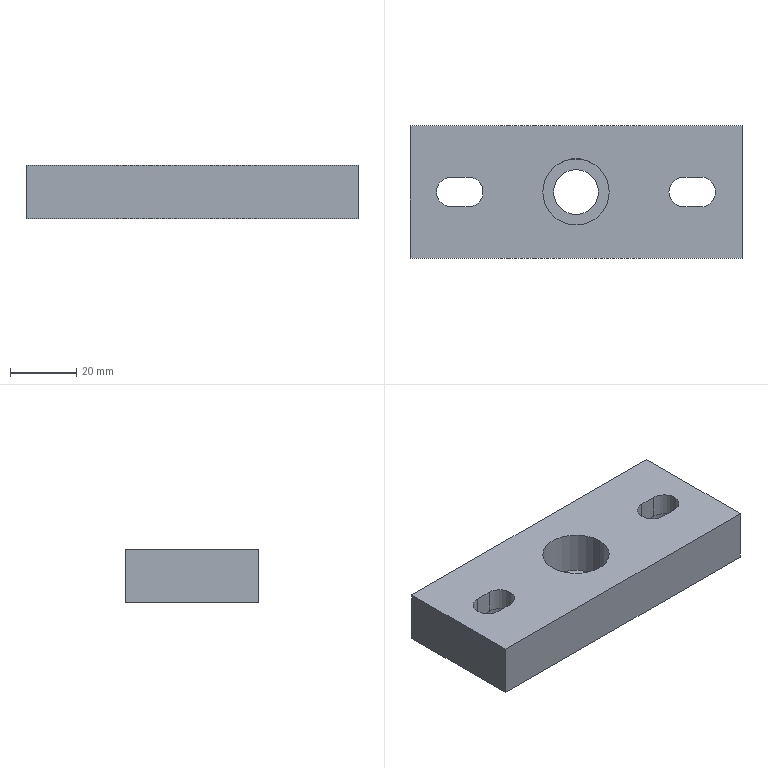Part | STEP file | X77b-01017 | 1 solid | 33 faces | box 100 x 40 x 16 mm | volume 53435 mm3 | plane 17 | cylinder 16 | commonest cylinder face diameters 9 x6 15 x6 13.5 x2 20 x2
STEP:
#1=CARTESIAN_POINT('',(10.527,125.181,9.));
#2=VERTEX_POINT('',#1);
#3=CARTESIAN_POINT('',(18.027,132.681,9.));
#4=VERTEX_POINT('',#3);
#5=CARTESIAN_POINT('',(18.027,125.181,9.));
#6=DIRECTION('',(0.,0.,-1.));
#7=DIRECTION('',(-1.,0.,0.));
#8=AXIS2_PLACEMENT_3D('',#5,#6,#7);
#9=CIRCLE('',#8,7.5);
#10=EDGE_CURVE('',#2,#4,#9,.T.);
#11=ORIENTED_EDGE('',*,*,#10,.F.);
#12=CARTESIAN_POINT('',(10.527,125.181,0.));
#13=VERTEX_POINT('',#12);
#14=CARTESIAN_POINT('',(10.527,125.181,9.));
#15=DIRECTION('',(0.,0.,-1.));
#16=VECTOR('',#15,1000.);
#17=LINE('',#14,#16);
#18=EDGE_CURVE('',#2,#13,#17,.T.);
#19=ORIENTED_EDGE('',*,*,#18,.T.);
#20=CARTESIAN_POINT('',(18.027,132.681,0.));
#21=VERTEX_POINT('',#20);
#22=CARTESIAN_POINT('',(18.027,125.181,0.));
#23=DIRECTION('',(0.,0.,-1.));
#24=DIRECTION('',(-1.,0.,0.));
#25=AXIS2_PLACEMENT_3D('',#22,#23,#24);
#26=CIRCLE('',#25,7.5);
#27=EDGE_CURVE('',#13,#21,#26,.T.);
#28=ORIENTED_EDGE('',*,*,#27,.T.);
#29=CARTESIAN_POINT('',(18.027,132.681,9.));
#30=DIRECTION('',(0.,0.,-1.));
#31=VECTOR('',#30,1000.);
#32=LINE('',#29,#31);
#33=EDGE_CURVE('',#4,#21,#32,.T.);
#34=ORIENTED_EDGE('',*,*,#33,.F.);
#35=EDGE_LOOP('',(#11,#19,#28,#34));
#36=FACE_OUTER_BOUND('',#35,.T.);
#37=CARTESIAN_POINT('',(18.027,125.181,9.));
#38=DIRECTION('',(0.,0.,-1.));
#39=DIRECTION('',(-1.,0.,0.));
#40=AXIS2_PLACEMENT_3D('',#37,#38,#39);
#41=CYLINDRICAL_SURFACE('',#40,7.5);
#42=ADVANCED_FACE('',(#36),#41,.F.);
#43=CARTESIAN_POINT('',(-59.473,125.181,9.));
#44=VERTEX_POINT('',#43);
#45=CARTESIAN_POINT('',(-51.973,132.681,9.));
#46=VERTEX_POINT('',#45);
#47=CARTESIAN_POINT('',(-51.973,125.181,9.));
#48=DIRECTION('',(0.,0.,-1.));
#49=DIRECTION('',(-1.,0.,0.));
#50=AXIS2_PLACEMENT_3D('',#47,#48,#49);
#51=CIRCLE('',#50,7.5);
#52=EDGE_CURVE('',#44,#46,#51,.T.);
#53=ORIENTED_EDGE('',*,*,#52,.F.);
#54=CARTESIAN_POINT('',(-59.473,125.181,0.));
#55=VERTEX_POINT('',#54);
#56=CARTESIAN_POINT('',(-59.473,125.181,9.));
#57=DIRECTION('',(0.,0.,-1.));
#58=VECTOR('',#57,1000.);
#59=LINE('',#56,#58);
#60=EDGE_CURVE('',#44,#55,#59,.T.);
#61=ORIENTED_EDGE('',*,*,#60,.T.);
#62=CARTESIAN_POINT('',(-51.973,132.681,0.));
#63=VERTEX_POINT('',#62);
#64=CARTESIAN_POINT('',(-51.973,125.181,0.));
#65=DIRECTION('',(0.,0.,-1.));
#66=DIRECTION('',(-1.,0.,0.));
#67=AXIS2_PLACEMENT_3D('',#64,#65,#66);
#68=CIRCLE('',#67,7.5);
#69=EDGE_CURVE('',#55,#63,#68,.T.);
#70=ORIENTED_EDGE('',*,*,#69,.T.);
#71=CARTESIAN_POINT('',(-51.973,132.681,9.));
#72=DIRECTION('',(0.,0.,-1.));
#73=VECTOR('',#72,1000.);
#74=LINE('',#71,#73);
#75=EDGE_CURVE('',#46,#63,#74,.T.);
#76=ORIENTED_EDGE('',*,*,#75,.F.);
#77=EDGE_LOOP('',(#53,#61,#70,#76));
#78=FACE_OUTER_BOUND('',#77,.T.);
#79=CARTESIAN_POINT('',(-51.973,125.181,9.));
#80=DIRECTION('',(0.,0.,-1.));
#81=DIRECTION('',(-1.,0.,0.));
#82=AXIS2_PLACEMENT_3D('',#79,#80,#81);
#83=CYLINDRICAL_SURFACE('',#82,7.5);
#84=ADVANCED_FACE('',(#78),#83,.F.);
#85=CARTESIAN_POINT('',(-24.473,125.181,3.));
#86=VERTEX_POINT('',#85);
#87=CARTESIAN_POINT('',(-4.473,125.181,3.));
#88=VERTEX_POINT('',#87);
#89=CARTESIAN_POINT('',(-14.473,125.181,3.));
#90=DIRECTION('',(0.,0.,1.));
#91=DIRECTION('',(1.,0.,0.));
#92=AXIS2_PLACEMENT_3D('',#89,#90,#91);
#93=CIRCLE('',#92,10.);
#94=EDGE_CURVE('',#86,#88,#93,.T.);
#95=ORIENTED_EDGE('',*,*,#94,.F.);
#96=CARTESIAN_POINT('',(-24.473,125.181,16.));
#97=VERTEX_POINT('',#96);
#98=CARTESIAN_POINT('',(-24.473,125.181,16.));
#99=DIRECTION('',(0.,0.,1.));
#100=VECTOR('',#99,1000.);
#101=LINE('',#98,#100);
#102=EDGE_CURVE('',#86,#97,#101,.T.);
#103=ORIENTED_EDGE('',*,*,#102,.T.);
#104=CARTESIAN_POINT('',(-4.473,125.181,16.));
#105=VERTEX_POINT('',#104);
#106=CARTESIAN_POINT('',(-14.473,125.181,16.));
#107=DIRECTION('',(0.,0.,1.));
#108=DIRECTION('',(1.,0.,0.));
#109=AXIS2_PLACEMENT_3D('',#106,#107,#108);
#110=CIRCLE('',#109,10.);
#111=EDGE_CURVE('',#97,#105,#110,.T.);
#112=ORIENTED_EDGE('',*,*,#111,.T.);
#113=CARTESIAN_POINT('',(-4.473,125.181,16.));
#114=DIRECTION('',(0.,0.,1.));
#115=VECTOR('',#114,1000.);
#116=LINE('',#113,#115);
#117=EDGE_CURVE('',#88,#105,#116,.T.);
#118=ORIENTED_EDGE('',*,*,#117,.F.);
#119=EDGE_LOOP('',(#95,#103,#112,#118));
#120=FACE_OUTER_BOUND('',#119,.T.);
#121=CARTESIAN_POINT('',(-14.473,125.181,16.));
#122=DIRECTION('',(0.,0.,1.));
#123=DIRECTION('',(1.,0.,0.));
#124=AXIS2_PLACEMENT_3D('',#121,#122,#123);
#125=CYLINDRICAL_SURFACE('',#124,10.);
#126=ADVANCED_FACE('',(#120),#125,.F.);
#127=CARTESIAN_POINT('',(-21.223,125.181,0.));
#128=VERTEX_POINT('',#127);
#129=CARTESIAN_POINT('',(-7.723,125.181,0.));
#130=VERTEX_POINT('',#129);
#131=CARTESIAN_POINT('',(-14.473,125.181,0.));
#132=DIRECTION('',(0.,0.,1.));
#133=DIRECTION('',(1.,0.,0.));
#134=AXIS2_PLACEMENT_3D('',#131,#132,#133);
#135=CIRCLE('',#134,6.75);
#136=EDGE_CURVE('',#128,#130,#135,.T.);
#137=ORIENTED_EDGE('',*,*,#136,.F.);
#138=CARTESIAN_POINT('',(-21.223,125.181,3.));
#139=VERTEX_POINT('',#138);
#140=CARTESIAN_POINT('',(-21.223,125.181,16.));
#141=DIRECTION('',(0.,0.,1.));
#142=VECTOR('',#141,1000.);
#143=LINE('',#140,#142);
#144=EDGE_CURVE('',#128,#139,#143,.T.);
#145=ORIENTED_EDGE('',*,*,#144,.T.);
#146=CARTESIAN_POINT('',(-7.723,125.181,3.));
#147=VERTEX_POINT('',#146);
#148=CARTESIAN_POINT('',(-14.473,125.181,3.));
#149=DIRECTION('',(0.,0.,1.));
#150=DIRECTION('',(1.,0.,0.));
#151=AXIS2_PLACEMENT_3D('',#148,#149,#150);
#152=CIRCLE('',#151,6.75);
#153=EDGE_CURVE('',#139,#147,#152,.T.);
#154=ORIENTED_EDGE('',*,*,#153,.T.);
#155=CARTESIAN_POINT('',(-7.723,125.181,16.));
#156=DIRECTION('',(0.,0.,1.));
#157=VECTOR('',#156,1000.);
#158=LINE('',#155,#157);
#159=EDGE_CURVE('',#130,#147,#158,.T.);
#160=ORIENTED_EDGE('',*,*,#159,.F.);
#161=EDGE_LOOP('',(#137,#145,#154,#160));
#162=FACE_OUTER_BOUND('',#161,.T.);
#163=CARTESIAN_POINT('',(-14.473,125.181,16.));
#164=DIRECTION('',(0.,0.,1.));
#165=DIRECTION('',(1.,0.,0.));
#166=AXIS2_PLACEMENT_3D('',#163,#164,#165);
#167=CYLINDRICAL_SURFACE('',#166,6.75);
#168=ADVANCED_FACE('',(#162),#167,.F.);
#169=CARTESIAN_POINT('',(-56.473,125.181,16.));
#170=VERTEX_POINT('',#169);
#171=CARTESIAN_POINT('',(-51.973,129.681,16.));
#172=VERTEX_POINT('',#171);
#173=CARTESIAN_POINT('',(-51.973,125.181,16.));
#174=DIRECTION('',(0.,0.,-1.));
#175=DIRECTION('',(-1.,0.,0.));
#176=AXIS2_PLACEMENT_3D('',#173,#174,#175);
#177=CIRCLE('',#176,4.5);
#178=EDGE_CURVE('',#170,#172,#177,.T.);
#179=ORIENTED_EDGE('',*,*,#178,.F.);
#180=CARTESIAN_POINT('',(-56.473,125.181,9.));
#181=VERTEX_POINT('',#180);
#182=CARTESIAN_POINT('',(-56.473,125.181,16.));
#183=DIRECTION('',(0.,0.,-1.));
#184=VECTOR('',#183,1000.);
#185=LINE('',#182,#184);
#186=EDGE_CURVE('',#170,#181,#185,.T.);
#187=ORIENTED_EDGE('',*,*,#186,.T.);
#188=CARTESIAN_POINT('',(-51.973,129.681,9.));
#189=VERTEX_POINT('',#188);
#190=CARTESIAN_POINT('',(-51.973,125.181,9.));
#191=DIRECTION('',(0.,0.,1.));
#192=DIRECTION('',(-1.,0.,0.));
#193=AXIS2_PLACEMENT_3D('',#190,#191,#192);
#194=CIRCLE('',#193,4.5);
#195=EDGE_CURVE('',#189,#181,#194,.T.);
#196=ORIENTED_EDGE('',*,*,#195,.F.);
#197=CARTESIAN_POINT('',(-51.973,129.681,16.));
#198=DIRECTION('',(0.,0.,-1.));
#199=VECTOR('',#198,1000.);
#200=LINE('',#197,#199);
#201=EDGE_CURVE('',#172,#189,#200,.T.);
#202=ORIENTED_EDGE('',*,*,#201,.F.);
#203=EDGE_LOOP('',(#179,#187,#196,#202));
#204=FACE_OUTER_BOUND('',#203,.T.);
#205=CARTESIAN_POINT('',(-51.973,125.181,16.));
#206=DIRECTION('',(0.,0.,-1.));
#207=DIRECTION('',(-1.,0.,0.));
#208=AXIS2_PLACEMENT_3D('',#205,#206,#207);
#209=CYLINDRICAL_SURFACE('',#208,4.5);
#210=ADVANCED_FACE('',(#204),#209,.F.);
#211=CARTESIAN_POINT('',(13.527,125.181,16.));
#212=VERTEX_POINT('',#211);
#213=CARTESIAN_POINT('',(18.027,129.681,16.));
#214=VERTEX_POINT('',#213);
#215=CARTESIAN_POINT('',(18.027,125.181,16.));
#216=DIRECTION('',(0.,0.,-1.));
#217=DIRECTION('',(-1.,0.,0.));
#218=AXIS2_PLACEMENT_3D('',#215,#216,#217);
#219=CIRCLE('',#218,4.5);
#220=EDGE_CURVE('',#212,#214,#219,.T.);
#221=ORIENTED_EDGE('',*,*,#220,.F.);
#222=CARTESIAN_POINT('',(13.527,125.181,9.));
#223=VERTEX_POINT('',#222);
#224=CARTESIAN_POINT('',(13.527,125.181,16.));
#225=DIRECTION('',(0.,0.,-1.));
#226=VECTOR('',#225,1000.);
#227=LINE('',#224,#226);
#228=EDGE_CURVE('',#212,#223,#227,.T.);
#229=ORIENTED_EDGE('',*,*,#228,.T.);
#230=CARTESIAN_POINT('',(18.027,129.681,9.));
#231=VERTEX_POINT('',#230);
#232=CARTESIAN_POINT('',(18.027,125.181,9.));
#233=DIRECTION('',(0.,0.,1.));
#234=DIRECTION('',(-1.,0.,0.));
#235=AXIS2_PLACEMENT_3D('',#232,#233,#234);
#236=CIRCLE('',#235,4.5);
#237=EDGE_CURVE('',#231,#223,#236,.T.);
#238=ORIENTED_EDGE('',*,*,#237,.F.);
#239=CARTESIAN_POINT('',(18.027,129.681,16.));
#240=DIRECTION('',(0.,0.,-1.));
#241=VECTOR('',#240,1000.);
#242=LINE('',#239,#241);
#243=EDGE_CURVE('',#214,#231,#242,.T.);
#244=ORIENTED_EDGE('',*,*,#243,.F.);
#245=EDGE_LOOP('',(#221,#229,#238,#244));
#246=FACE_OUTER_BOUND('',#245,.T.);
#247=CARTESIAN_POINT('',(18.027,125.181,16.));
#248=DIRECTION('',(0.,0.,-1.));
#249=DIRECTION('',(-1.,0.,0.));
#250=AXIS2_PLACEMENT_3D('',#247,#248,#249);
#251=CYLINDRICAL_SURFACE('',#250,4.5);
#252=ADVANCED_FACE('',(#246),#251,.F.);
#253=CARTESIAN_POINT('',(23.027,120.681,9.));
#254=VERTEX_POINT('',#253);
#255=CARTESIAN_POINT('',(23.027,129.681,9.));
#256=VERTEX_POINT('',#255);
#257=CARTESIAN_POINT('',(23.027,125.181,9.));
#258=DIRECTION('',(0.,0.,1.));
#259=DIRECTION('',(-1.,0.,0.));
#260=AXIS2_PLACEMENT_3D('',#257,#258,#259);
#261=CIRCLE('',#260,4.5);
#262=EDGE_CURVE('',#254,#256,#261,.T.);
#263=ORIENTED_EDGE('',*,*,#262,.F.);
#264=CARTESIAN_POINT('',(23.027,120.681,16.));
#265=VERTEX_POINT('',#264);
#266=CARTESIAN_POINT('',(23.027,120.681,16.));
#267=DIRECTION('',(0.,0.,-1.));
#268=VECTOR('',#267,1000.);
#269=LINE('',#266,#268);
#270=EDGE_CURVE('',#265,#254,#269,.T.);
#271=ORIENTED_EDGE('',*,*,#270,.F.);
#272=CARTESIAN_POINT('',(23.027,129.681,16.));
#273=VERTEX_POINT('',#272);
#274=CARTESIAN_POINT('',(23.027,125.181,16.));
#275=DIRECTION('',(0.,0.,-1.));
#276=DIRECTION('',(-1.,0.,0.));
#277=AXIS2_PLACEMENT_3D('',#274,#275,#276);
#278=CIRCLE('',#277,4.5);
#279=EDGE_CURVE('',#273,#265,#278,.T.);
#280=ORIENTED_EDGE('',*,*,#279,.F.);
#281=CARTESIAN_POINT('',(23.027,129.681,16.));
#282=DIRECTION('',(0.,0.,-1.));
#283=VECTOR('',#282,1000.);
#284=LINE('',#281,#283);
#285=EDGE_CURVE('',#273,#256,#284,.T.);
#286=ORIENTED_EDGE('',*,*,#285,.T.);
#287=EDGE_LOOP('',(#263,#271,#280,#286));
#288=FACE_OUTER_BOUND('',#287,.T.);
#289=CARTESIAN_POINT('',(23.027,125.181,16.));
#290=DIRECTION('',(0.,0.,-1.));
#291=DIRECTION('',(-1.,0.,0.));
#292=AXIS2_PLACEMENT_3D('',#289,#290,#291);
#293=CYLINDRICAL_SURFACE('',#292,4.5);
#294=ADVANCED_FACE('',(#288),#293,.F.);
#295=CARTESIAN_POINT('',(23.027,129.681,9.));
#296=DIRECTION('',(-1.,0.,0.));
#297=VECTOR('',#296,1000.);
#298=LINE('',#295,#297);
#299=EDGE_CURVE('',#256,#231,#298,.T.);
#300=ORIENTED_EDGE('',*,*,#299,.F.);
#301=ORIENTED_EDGE('',*,*,#285,.F.);
#302=CARTESIAN_POINT('',(23.027,129.681,16.));
#303=DIRECTION('',(1.,0.,0.));
#304=VECTOR('',#303,1000.);
#305=LINE('',#302,#304);
#306=EDGE_CURVE('',#214,#273,#305,.T.);
#307=ORIENTED_EDGE('',*,*,#306,.F.);
#308=ORIENTED_EDGE('',*,*,#243,.T.);
#309=EDGE_LOOP('',(#300,#301,#307,#308));
#310=FACE_OUTER_BOUND('',#309,.T.);
#311=CARTESIAN_POINT('',(23.027,129.681,16.));
#312=DIRECTION('',(0.,1.,0.));
#313=DIRECTION('',(0.,0.,1.));
#314=AXIS2_PLACEMENT_3D('',#311,#312,#313);
#315=PLANE('',#314);
#316=ADVANCED_FACE('',(#310),#315,.F.);
#317=ORIENTED_EDGE('',*,*,#228,.F.);
#318=CARTESIAN_POINT('',(18.027,120.681,16.));
#319=VERTEX_POINT('',#318);
#320=CARTESIAN_POINT('',(18.027,125.181,16.));
#321=DIRECTION('',(0.,0.,-1.));
#322=DIRECTION('',(-1.,0.,0.));
#323=AXIS2_PLACEMENT_3D('',#320,#321,#322);
#324=CIRCLE('',#323,4.5);
#325=EDGE_CURVE('',#319,#212,#324,.T.);
#326=ORIENTED_EDGE('',*,*,#325,.F.);
#327=CARTESIAN_POINT('',(18.027,120.681,9.));
#328=VERTEX_POINT('',#327);
#329=CARTESIAN_POINT('',(18.027,120.681,16.));
#330=DIRECTION('',(0.,0.,-1.));
#331=VECTOR('',#330,1000.);
#332=LINE('',#329,#331);
#333=EDGE_CURVE('',#319,#328,#332,.T.);
#334=ORIENTED_EDGE('',*,*,#333,.T.);
#335=CARTESIAN_POINT('',(18.027,125.181,9.));
#336=DIRECTION('',(0.,0.,1.));
#337=DIRECTION('',(-1.,0.,0.));
#338=AXIS2_PLACEMENT_3D('',#335,#336,#337);
#339=CIRCLE('',#338,4.5);
#340=EDGE_CURVE('',#223,#328,#339,.T.);
#341=ORIENTED_EDGE('',*,*,#340,.F.);
#342=EDGE_LOOP('',(#317,#326,#334,#341));
#343=FACE_OUTER_BOUND('',#342,.T.);
#344=CARTESIAN_POINT('',(18.027,125.181,16.));
#345=DIRECTION('',(0.,0.,-1.));
#346=DIRECTION('',(-1.,0.,0.));
#347=AXIS2_PLACEMENT_3D('',#344,#345,#346);
#348=CYLINDRICAL_SURFACE('',#347,4.5);
#349=ADVANCED_FACE('',(#343),#348,.F.);
#350=CARTESIAN_POINT('',(23.027,120.681,9.));
#351=DIRECTION('',(1.,0.,0.));
#352=VECTOR('',#351,1000.);
#353=LINE('',#350,#352);
#354=EDGE_CURVE('',#328,#254,#353,.T.);
#355=ORIENTED_EDGE('',*,*,#354,.F.);
#356=ORIENTED_EDGE('',*,*,#333,.F.);
#357=CARTESIAN_POINT('',(23.027,120.681,16.));
#358=DIRECTION('',(-1.,0.,0.));
#359=VECTOR('',#358,1000.);
#360=LINE('',#357,#359);
#361=EDGE_CURVE('',#265,#319,#360,.T.);
#362=ORIENTED_EDGE('',*,*,#361,.F.);
#363=ORIENTED_EDGE('',*,*,#270,.T.);
#364=EDGE_LOOP('',(#355,#356,#362,#363));
#365=FACE_OUTER_BOUND('',#364,.T.);
#366=CARTESIAN_POINT('',(23.027,120.681,16.));
#367=DIRECTION('',(0.,-1.,0.));
#368=DIRECTION('',(0.,0.,-1.));
#369=AXIS2_PLACEMENT_3D('',#366,#367,#368);
#370=PLANE('',#369);
#371=ADVANCED_FACE('',(#365),#370,.F.);
#372=CARTESIAN_POINT('',(-46.973,120.681,9.));
#373=VERTEX_POINT('',#372);
#374=CARTESIAN_POINT('',(-46.973,129.681,9.));
#375=VERTEX_POINT('',#374);
#376=CARTESIAN_POINT('',(-46.973,125.181,9.));
#377=DIRECTION('',(0.,0.,1.));
#378=DIRECTION('',(-1.,0.,0.));
#379=AXIS2_PLACEMENT_3D('',#376,#377,#378);
#380=CIRCLE('',#379,4.5);
#381=EDGE_CURVE('',#373,#375,#380,.T.);
#382=ORIENTED_EDGE('',*,*,#381,.F.);
#383=CARTESIAN_POINT('',(-46.973,120.681,16.));
#384=VERTEX_POINT('',#383);
#385=CARTESIAN_POINT('',(-46.973,120.681,16.));
#386=DIRECTION('',(0.,0.,-1.));
#387=VECTOR('',#386,1000.);
#388=LINE('',#385,#387);
#389=EDGE_CURVE('',#384,#373,#388,.T.);
#390=ORIENTED_EDGE('',*,*,#389,.F.);
#391=CARTESIAN_POINT('',(-46.973,129.681,16.));
#392=VERTEX_POINT('',#391);
#393=CARTESIAN_POINT('',(-46.973,125.181,16.));
#394=DIRECTION('',(0.,0.,-1.));
#395=DIRECTION('',(-1.,0.,0.));
#396=AXIS2_PLACEMENT_3D('',#393,#394,#395);
#397=CIRCLE('',#396,4.5);
#398=EDGE_CURVE('',#392,#384,#397,.T.);
#399=ORIENTED_EDGE('',*,*,#398,.F.);
#400=CARTESIAN_POINT('',(-46.973,129.681,16.));
#401=DIRECTION('',(0.,0.,-1.));
#402=VECTOR('',#401,1000.);
#403=LINE('',#400,#402);
#404=EDGE_CURVE('',#392,#375,#403,.T.);
#405=ORIENTED_EDGE('',*,*,#404,.T.);
#406=EDGE_LOOP('',(#382,#390,#399,#405));
#407=FACE_OUTER_BOUND('',#406,.T.);
#408=CARTESIAN_POINT('',(-46.973,125.181,16.));
#409=DIRECTION('',(0.,0.,-1.));
#410=DIRECTION('',(-1.,0.,0.));
#411=AXIS2_PLACEMENT_3D('',#408,#409,#410);
#412=CYLINDRICAL_SURFACE('',#411,4.5);
#413=ADVANCED_FACE('',(#407),#412,.F.);
#414=CARTESIAN_POINT('',(-46.973,129.681,9.));
#415=DIRECTION('',(-1.,0.,0.));
#416=VECTOR('',#415,1000.);
#417=LINE('',#414,#416);
#418=EDGE_CURVE('',#375,#189,#417,.T.);
#419=ORIENTED_EDGE('',*,*,#418,.F.);
#420=ORIENTED_EDGE('',*,*,#404,.F.);
#421=CARTESIAN_POINT('',(-46.973,129.681,16.));
#422=DIRECTION('',(1.,0.,0.));
#423=VECTOR('',#422,1000.);
#424=LINE('',#421,#423);
#425=EDGE_CURVE('',#172,#392,#424,.T.);
#426=ORIENTED_EDGE('',*,*,#425,.F.);
#427=ORIENTED_EDGE('',*,*,#201,.T.);
#428=EDGE_LOOP('',(#419,#420,#426,#427));
#429=FACE_OUTER_BOUND('',#428,.T.);
#430=CARTESIAN_POINT('',(-46.973,129.681,16.));
#431=DIRECTION('',(0.,1.,0.));
#432=DIRECTION('',(0.,0.,1.));
#433=AXIS2_PLACEMENT_3D('',#430,#431,#432);
#434=PLANE('',#433);
#435=ADVANCED_FACE('',(#429),#434,.F.);
#436=ORIENTED_EDGE('',*,*,#186,.F.);
#437=CARTESIAN_POINT('',(-51.973,120.681,16.));
#438=VERTEX_POINT('',#437);
#439=CARTESIAN_POINT('',(-51.973,125.181,16.));
#440=DIRECTION('',(0.,0.,-1.));
#441=DIRECTION('',(-1.,0.,0.));
#442=AXIS2_PLACEMENT_3D('',#439,#440,#441);
#443=CIRCLE('',#442,4.5);
#444=EDGE_CURVE('',#438,#170,#443,.T.);
#445=ORIENTED_EDGE('',*,*,#444,.F.);
#446=CARTESIAN_POINT('',(-51.973,120.681,9.));
#447=VERTEX_POINT('',#446);
#448=CARTESIAN_POINT('',(-51.973,120.681,16.));
#449=DIRECTION('',(0.,0.,-1.));
#450=VECTOR('',#449,1000.);
#451=LINE('',#448,#450);
#452=EDGE_CURVE('',#438,#447,#451,.T.);
#453=ORIENTED_EDGE('',*,*,#452,.T.);
#454=CARTESIAN_POINT('',(-51.973,125.181,9.));
#455=DIRECTION('',(0.,0.,1.));
#456=DIRECTION('',(-1.,0.,0.));
#457=AXIS2_PLACEMENT_3D('',#454,#455,#456);
#458=CIRCLE('',#457,4.5);
#459=EDGE_CURVE('',#181,#447,#458,.T.);
#460=ORIENTED_EDGE('',*,*,#459,.F.);
#461=EDGE_LOOP('',(#436,#445,#453,#460));
#462=FACE_OUTER_BOUND('',#461,.T.);
#463=CARTESIAN_POINT('',(-51.973,125.181,16.));
#464=DIRECTION('',(0.,0.,-1.));
#465=DIRECTION('',(-1.,0.,0.));
#466=AXIS2_PLACEMENT_3D('',#463,#464,#465);
#467=CYLINDRICAL_SURFACE('',#466,4.5);
#468=ADVANCED_FACE('',(#462),#467,.F.);
#469=CARTESIAN_POINT('',(-46.973,120.681,9.));
#470=DIRECTION('',(1.,0.,0.));
#471=VECTOR('',#470,1000.);
#472=LINE('',#469,#471);
#473=EDGE_CURVE('',#447,#373,#472,.T.);
#474=ORIENTED_EDGE('',*,*,#473,.F.);
#475=ORIENTED_EDGE('',*,*,#452,.F.);
#476=CARTESIAN_POINT('',(-46.973,120.681,16.));
#477=DIRECTION('',(-1.,0.,0.));
#478=VECTOR('',#477,1000.);
#479=LINE('',#476,#478);
#480=EDGE_CURVE('',#384,#438,#479,.T.);
#481=ORIENTED_EDGE('',*,*,#480,.F.);
#482=ORIENTED_EDGE('',*,*,#389,.T.);
#483=EDGE_LOOP('',(#474,#475,#481,#482));
#484=FACE_OUTER_BOUND('',#483,.T.);
#485=CARTESIAN_POINT('',(-46.973,120.681,16.));
#486=DIRECTION('',(0.,-1.,0.));
#487=DIRECTION('',(0.,0.,-1.));
#488=AXIS2_PLACEMENT_3D('',#485,#486,#487);
#489=PLANE('',#488);
#490=ADVANCED_FACE('',(#484),#489,.F.);
#491=CARTESIAN_POINT('',(-64.473,145.181,0.));
#492=VERTEX_POINT('',#491);
#493=CARTESIAN_POINT('',(-64.473,105.181,0.));
#494=VERTEX_POINT('',#493);
#495=CARTESIAN_POINT('',(-64.473,105.181,0.));
#496=DIRECTION('',(0.,-1.,0.));
#497=VECTOR('',#496,1000.);
#498=LINE('',#495,#497);
#499=EDGE_CURVE('',#492,#494,#498,.T.);
#500=ORIENTED_EDGE('',*,*,#499,.T.);
#501=CARTESIAN_POINT('',(-64.473,105.181,16.));
#502=VERTEX_POINT('',#501);
#503=CARTESIAN_POINT('',(-64.473,105.181,16.));
#504=DIRECTION('',(0.,0.,-1.));
#505=VECTOR('',#504,1000.);
#506=LINE('',#503,#505);
#507=EDGE_CURVE('',#502,#494,#506,.T.);
#508=ORIENTED_EDGE('',*,*,#507,.F.);
#509=CARTESIAN_POINT('',(-64.473,145.181,16.));
#510=VERTEX_POINT('',#509);
#511=CARTESIAN_POINT('',(-64.473,105.181,16.));
#512=DIRECTION('',(0.,-1.,0.));
#513=VECTOR('',#512,1000.);
#514=LINE('',#511,#513);
#515=EDGE_CURVE('',#510,#502,#514,.T.);
#516=ORIENTED_EDGE('',*,*,#515,.F.);
#517=CARTESIAN_POINT('',(-64.473,145.181,16.));
#518=DIRECTION('',(0.,0.,-1.));
#519=VECTOR('',#518,1000.);
#520=LINE('',#517,#519);
#521=EDGE_CURVE('',#510,#492,#520,.T.);
#522=ORIENTED_EDGE('',*,*,#521,.T.);
#523=EDGE_LOOP('',(#500,#508,#516,#522));
#524=FACE_OUTER_BOUND('',#523,.T.);
#525=CARTESIAN_POINT('',(-64.473,105.181,16.));
#526=DIRECTION('',(1.,0.,0.));
#527=DIRECTION('',(0.,0.,-1.));
#528=AXIS2_PLACEMENT_3D('',#525,#526,#527);
#529=PLANE('',#528);
#530=ADVANCED_FACE('',(#524),#529,.F.);
#531=CARTESIAN_POINT('',(35.527,105.181,0.));
#532=VERTEX_POINT('',#531);
#533=CARTESIAN_POINT('',(-64.473,105.181,0.));
#534=DIRECTION('',(1.,0.,0.));
#535=VECTOR('',#534,1000.);
#536=LINE('',#533,#535);
#537=EDGE_CURVE('',#494,#532,#536,.T.);
#538=ORIENTED_EDGE('',*,*,#537,.T.);
#539=CARTESIAN_POINT('',(35.527,105.181,16.));
#540=VERTEX_POINT('',#539);
#541=CARTESIAN_POINT('',(35.527,105.181,16.));
#542=DIRECTION('',(0.,0.,-1.));
#543=VECTOR('',#542,1000.);
#544=LINE('',#541,#543);
#545=EDGE_CURVE('',#540,#532,#544,.T.);
#546=ORIENTED_EDGE('',*,*,#545,.F.);
#547=CARTESIAN_POINT('',(-64.473,105.181,16.));
#548=DIRECTION('',(1.,0.,0.));
#549=VECTOR('',#548,1000.);
#550=LINE('',#547,#549);
#551=EDGE_CURVE('',#502,#540,#550,.T.);
#552=ORIENTED_EDGE('',*,*,#551,.F.);
#553=ORIENTED_EDGE('',*,*,#507,.T.);
#554=EDGE_LOOP('',(#538,#546,#552,#553));
#555=FACE_OUTER_BOUND('',#554,.T.);
#556=CARTESIAN_POINT('',(-64.473,105.181,16.));
#557=DIRECTION('',(0.,1.,0.));
#558=DIRECTION('',(0.,0.,1.));
#559=AXIS2_PLACEMENT_3D('',#556,#557,#558);
#560=PLANE('',#559);
#561=ADVANCED_FACE('',(#555),#560,.F.);
#562=CARTESIAN_POINT('',(35.527,145.181,0.));
#563=VERTEX_POINT('',#562);
#564=CARTESIAN_POINT('',(35.527,105.181,0.));
#565=DIRECTION('',(0.,1.,0.));
#566=VECTOR('',#565,1000.);
#567=LINE('',#564,#566);
#568=EDGE_CURVE('',#532,#563,#567,.T.);
#569=ORIENTED_EDGE('',*,*,#568,.T.);
#570=CARTESIAN_POINT('',(35.527,145.181,16.));
#571=VERTEX_POINT('',#570);
#572=CARTESIAN_POINT('',(35.527,145.181,16.));
#573=DIRECTION('',(0.,0.,-1.));
#574=VECTOR('',#573,1000.);
#575=LINE('',#572,#574);
#576=EDGE_CURVE('',#571,#563,#575,.T.);
#577=ORIENTED_EDGE('',*,*,#576,.F.);
#578=CARTESIAN_POINT('',(35.527,105.181,16.));
#579=DIRECTION('',(0.,1.,0.));
#580=VECTOR('',#579,1000.);
#581=LINE('',#578,#580);
#582=EDGE_CURVE('',#540,#571,#581,.T.);
#583=ORIENTED_EDGE('',*,*,#582,.F.);
#584=ORIENTED_EDGE('',*,*,#545,.T.);
#585=EDGE_LOOP('',(#569,#577,#583,#584));
#586=FACE_OUTER_BOUND('',#585,.T.);
#587=CARTESIAN_POINT('',(35.527,105.181,16.));
#588=DIRECTION('',(-1.,0.,0.));
#589=DIRECTION('',(0.,0.,1.));
#590=AXIS2_PLACEMENT_3D('',#587,#588,#589);
#591=PLANE('',#590);
#592=ADVANCED_FACE('',(#586),#591,.F.);
#593=CARTESIAN_POINT('',(-64.473,145.181,0.));
#594=DIRECTION('',(-1.,0.,0.));
#595=VECTOR('',#594,1000.);
#596=LINE('',#593,#595);
#597=EDGE_CURVE('',#563,#492,#596,.T.);
#598=ORIENTED_EDGE('',*,*,#597,.T.);
#599=ORIENTED_EDGE('',*,*,#521,.F.);
#600=CARTESIAN_POINT('',(-64.473,145.181,16.));
#601=DIRECTION('',(-1.,0.,0.));
#602=VECTOR('',#601,1000.);
#603=LINE('',#600,#602);
#604=EDGE_CURVE('',#571,#510,#603,.T.);
#605=ORIENTED_EDGE('',*,*,#604,.F.);
#606=ORIENTED_EDGE('',*,*,#576,.T.);
#607=EDGE_LOOP('',(#598,#599,#605,#606));
#608=FACE_OUTER_BOUND('',#607,.T.);
#609=CARTESIAN_POINT('',(-64.473,145.181,16.));
#610=DIRECTION('',(0.,-1.,0.));
#611=DIRECTION('',(0.,0.,-1.));
#612=AXIS2_PLACEMENT_3D('',#609,#610,#611);
#613=PLANE('',#612);
#614=ADVANCED_FACE('',(#608),#613,.F.);
#615=ORIENTED_EDGE('',*,*,#425,.T.);
#616=ORIENTED_EDGE('',*,*,#398,.T.);
#617=ORIENTED_EDGE('',*,*,#480,.T.);
#618=ORIENTED_EDGE('',*,*,#444,.T.);
#619=ORIENTED_EDGE('',*,*,#178,.T.);
#620=EDGE_LOOP('',(#615,#616,#617,#618,#619));
#621=FACE_BOUND('',#620,.T.);
#622=ORIENTED_EDGE('',*,*,#306,.T.);
#623=ORIENTED_EDGE('',*,*,#279,.T.);
#624=ORIENTED_EDGE('',*,*,#361,.T.);
#625=ORIENTED_EDGE('',*,*,#325,.T.);
#626=ORIENTED_EDGE('',*,*,#220,.T.);
#627=EDGE_LOOP('',(#622,#623,#624,#625,#626));
#628=FACE_BOUND('',#627,.T.);
#629=CARTESIAN_POINT('',(-14.473,125.181,16.));
#630=DIRECTION('',(0.,0.,1.));
#631=DIRECTION('',(1.,0.,0.));
#632=AXIS2_PLACEMENT_3D('',#629,#630,#631);
#633=CIRCLE('',#632,10.);
#634=EDGE_CURVE('',#105,#97,#633,.T.);
#635=ORIENTED_EDGE('',*,*,#634,.F.);
#636=ORIENTED_EDGE('',*,*,#111,.F.);
#637=EDGE_LOOP('',(#635,#636));
#638=FACE_BOUND('',#637,.T.);
#639=ORIENTED_EDGE('',*,*,#515,.T.);
#640=ORIENTED_EDGE('',*,*,#551,.T.);
#641=ORIENTED_EDGE('',*,*,#582,.T.);
#642=ORIENTED_EDGE('',*,*,#604,.T.);
#643=EDGE_LOOP('',(#639,#640,#641,#642));
#644=FACE_OUTER_BOUND('',#643,.T.);
#645=CARTESIAN_POINT('',(-64.473,145.181,16.));
#646=DIRECTION('',(0.,0.,-1.));
#647=DIRECTION('',(-1.,0.,0.));
#648=AXIS2_PLACEMENT_3D('',#645,#646,#647);
#649=PLANE('',#648);
#650=ADVANCED_FACE('',(#621,#628,#638,#644),#649,.F.);
#651=CARTESIAN_POINT('',(18.027,117.681,0.));
#652=VERTEX_POINT('',#651);
#653=CARTESIAN_POINT('',(18.027,125.181,0.));
#654=DIRECTION('',(0.,0.,-1.));
#655=DIRECTION('',(-1.,0.,0.));
#656=AXIS2_PLACEMENT_3D('',#653,#654,#655);
#657=CIRCLE('',#656,7.5);
#658=EDGE_CURVE('',#652,#13,#657,.T.);
#659=ORIENTED_EDGE('',*,*,#658,.F.);
#660=CARTESIAN_POINT('',(23.027,117.681,0.));
#661=VERTEX_POINT('',#660);
#662=CARTESIAN_POINT('',(23.027,117.681,0.));
#663=DIRECTION('',(-1.,0.,0.));
#664=VECTOR('',#663,1000.);
#665=LINE('',#662,#664);
#666=EDGE_CURVE('',#661,#652,#665,.T.);
#667=ORIENTED_EDGE('',*,*,#666,.F.);
#668=CARTESIAN_POINT('',(23.027,132.681,0.));
#669=VERTEX_POINT('',#668);
#670=CARTESIAN_POINT('',(23.027,125.181,0.));
#671=DIRECTION('',(0.,0.,-1.));
#672=DIRECTION('',(-1.,0.,0.));
#673=AXIS2_PLACEMENT_3D('',#670,#671,#672);
#674=CIRCLE('',#673,7.5);
#675=EDGE_CURVE('',#669,#661,#674,.T.);
#676=ORIENTED_EDGE('',*,*,#675,.F.);
#677=CARTESIAN_POINT('',(18.027,132.681,0.));
#678=DIRECTION('',(1.,0.,0.));
#679=VECTOR('',#678,1000.);
#680=LINE('',#677,#679);
#681=EDGE_CURVE('',#21,#669,#680,.T.);
#682=ORIENTED_EDGE('',*,*,#681,.F.);
#683=ORIENTED_EDGE('',*,*,#27,.F.);
#684=EDGE_LOOP('',(#659,#667,#676,#682,#683));
#685=FACE_BOUND('',#684,.T.);
#686=CARTESIAN_POINT('',(-51.973,117.681,0.));
#687=VERTEX_POINT('',#686);
#688=CARTESIAN_POINT('',(-51.973,125.181,0.));
#689=DIRECTION('',(0.,0.,-1.));
#690=DIRECTION('',(-1.,0.,0.));
#691=AXIS2_PLACEMENT_3D('',#688,#689,#690);
#692=CIRCLE('',#691,7.5);
#693=EDGE_CURVE('',#687,#55,#692,.T.);
#694=ORIENTED_EDGE('',*,*,#693,.F.);
#695=CARTESIAN_POINT('',(-46.973,117.681,0.));
#696=VERTEX_POINT('',#695);
#697=CARTESIAN_POINT('',(-46.973,117.681,0.));
#698=DIRECTION('',(-1.,0.,0.));
#699=VECTOR('',#698,1000.);
#700=LINE('',#697,#699);
#701=EDGE_CURVE('',#696,#687,#700,.T.);
#702=ORIENTED_EDGE('',*,*,#701,.F.);
#703=CARTESIAN_POINT('',(-46.973,132.681,0.));
#704=VERTEX_POINT('',#703);
#705=CARTESIAN_POINT('',(-46.973,125.181,0.));
#706=DIRECTION('',(0.,0.,-1.));
#707=DIRECTION('',(-1.,0.,0.));
#708=AXIS2_PLACEMENT_3D('',#705,#706,#707);
#709=CIRCLE('',#708,7.5);
#710=EDGE_CURVE('',#704,#696,#709,.T.);
#711=ORIENTED_EDGE('',*,*,#710,.F.);
#712=CARTESIAN_POINT('',(-51.973,132.681,0.));
#713=DIRECTION('',(1.,0.,0.));
#714=VECTOR('',#713,1000.);
#715=LINE('',#712,#714);
#716=EDGE_CURVE('',#63,#704,#715,.T.);
#717=ORIENTED_EDGE('',*,*,#716,.F.);
#718=ORIENTED_EDGE('',*,*,#69,.F.);
#719=EDGE_LOOP('',(#694,#702,#711,#717,#718));
#720=FACE_BOUND('',#719,.T.);
#721=CARTESIAN_POINT('',(-14.473,125.181,0.));
#722=DIRECTION('',(0.,0.,1.));
#723=DIRECTION('',(1.,0.,0.));
#724=AXIS2_PLACEMENT_3D('',#721,#722,#723);
#725=CIRCLE('',#724,6.75);
#726=EDGE_CURVE('',#130,#128,#725,.T.);
#727=ORIENTED_EDGE('',*,*,#726,.T.);
#728=ORIENTED_EDGE('',*,*,#136,.T.);
#729=EDGE_LOOP('',(#727,#728));
#730=FACE_BOUND('',#729,.T.);
#731=ORIENTED_EDGE('',*,*,#499,.F.);
#732=ORIENTED_EDGE('',*,*,#597,.F.);
#733=ORIENTED_EDGE('',*,*,#568,.F.);
#734=ORIENTED_EDGE('',*,*,#537,.F.);
#735=EDGE_LOOP('',(#731,#732,#733,#734));
#736=FACE_OUTER_BOUND('',#735,.T.);
#737=CARTESIAN_POINT('',(-64.473,145.181,0.));
#738=DIRECTION('',(0.,0.,-1.));
#739=DIRECTION('',(-1.,0.,0.));
#740=AXIS2_PLACEMENT_3D('',#737,#738,#739);
#741=PLANE('',#740);
#742=ADVANCED_FACE('',(#685,#720,#730,#736),#741,.T.);
#743=ORIENTED_EDGE('',*,*,#144,.F.);
#744=ORIENTED_EDGE('',*,*,#726,.F.);
#745=ORIENTED_EDGE('',*,*,#159,.T.);
#746=CARTESIAN_POINT('',(-14.473,125.181,3.));
#747=DIRECTION('',(0.,0.,1.));
#748=DIRECTION('',(1.,0.,0.));
#749=AXIS2_PLACEMENT_3D('',#746,#747,#748);
#750=CIRCLE('',#749,6.75);
#751=EDGE_CURVE('',#147,#139,#750,.T.);
#752=ORIENTED_EDGE('',*,*,#751,.T.);
#753=EDGE_LOOP('',(#743,#744,#745,#752));
#754=FACE_OUTER_BOUND('',#753,.T.);
#755=CARTESIAN_POINT('',(-14.473,125.181,16.));
#756=DIRECTION('',(0.,0.,1.));
#757=DIRECTION('',(1.,0.,0.));
#758=AXIS2_PLACEMENT_3D('',#755,#756,#757);
#759=CYLINDRICAL_SURFACE('',#758,6.75);
#760=ADVANCED_FACE('',(#754),#759,.F.);
#761=ORIENTED_EDGE('',*,*,#751,.F.);
#762=ORIENTED_EDGE('',*,*,#153,.F.);
#763=EDGE_LOOP('',(#761,#762));
#764=FACE_BOUND('',#763,.T.);
#765=CARTESIAN_POINT('',(-14.473,125.181,3.));
#766=DIRECTION('',(0.,0.,1.));
#767=DIRECTION('',(1.,0.,0.));
#768=AXIS2_PLACEMENT_3D('',#765,#766,#767);
#769=CIRCLE('',#768,10.);
#770=EDGE_CURVE('',#88,#86,#769,.T.);
#771=ORIENTED_EDGE('',*,*,#770,.T.);
#772=ORIENTED_EDGE('',*,*,#94,.T.);
#773=EDGE_LOOP('',(#771,#772));
#774=FACE_OUTER_BOUND('',#773,.T.);
#775=CARTESIAN_POINT('',(-7.723,125.181,3.));
#776=DIRECTION('',(0.,0.,-1.));
#777=DIRECTION('',(-1.,0.,0.));
#778=AXIS2_PLACEMENT_3D('',#775,#776,#777);
#779=PLANE('',#778);
#780=ADVANCED_FACE('',(#764,#774),#779,.F.);
#781=ORIENTED_EDGE('',*,*,#102,.F.);
#782=ORIENTED_EDGE('',*,*,#770,.F.);
#783=ORIENTED_EDGE('',*,*,#117,.T.);
#784=ORIENTED_EDGE('',*,*,#634,.T.);
#785=EDGE_LOOP('',(#781,#782,#783,#784));
#786=FACE_OUTER_BOUND('',#785,.T.);
#787=CARTESIAN_POINT('',(-14.473,125.181,16.));
#788=DIRECTION('',(0.,0.,1.));
#789=DIRECTION('',(1.,0.,0.));
#790=AXIS2_PLACEMENT_3D('',#787,#788,#789);
#791=CYLINDRICAL_SURFACE('',#790,10.);
#792=ADVANCED_FACE('',(#786),#791,.F.);
#793=CARTESIAN_POINT('',(-51.973,117.681,9.));
#794=VERTEX_POINT('',#793);
#795=CARTESIAN_POINT('',(-51.973,125.181,9.));
#796=DIRECTION('',(0.,0.,-1.));
#797=DIRECTION('',(-1.,0.,0.));
#798=AXIS2_PLACEMENT_3D('',#795,#796,#797);
#799=CIRCLE('',#798,7.5);
#800=EDGE_CURVE('',#794,#44,#799,.T.);
#801=ORIENTED_EDGE('',*,*,#800,.T.);
#802=ORIENTED_EDGE('',*,*,#52,.T.);
#803=CARTESIAN_POINT('',(-46.973,132.681,9.));
#804=VERTEX_POINT('',#803);
#805=CARTESIAN_POINT('',(-51.973,132.681,9.));
#806=DIRECTION('',(1.,0.,0.));
#807=VECTOR('',#806,1000.);
#808=LINE('',#805,#807);
#809=EDGE_CURVE('',#46,#804,#808,.T.);
#810=ORIENTED_EDGE('',*,*,#809,.T.);
#811=CARTESIAN_POINT('',(-46.973,117.681,9.));
#812=VERTEX_POINT('',#811);
#813=CARTESIAN_POINT('',(-46.973,125.181,9.));
#814=DIRECTION('',(0.,0.,-1.));
#815=DIRECTION('',(-1.,0.,0.));
#816=AXIS2_PLACEMENT_3D('',#813,#814,#815);
#817=CIRCLE('',#816,7.5);
#818=EDGE_CURVE('',#804,#812,#817,.T.);
#819=ORIENTED_EDGE('',*,*,#818,.T.);
#820=CARTESIAN_POINT('',(-46.973,117.681,9.));
#821=DIRECTION('',(-1.,0.,0.));
#822=VECTOR('',#821,1000.);
#823=LINE('',#820,#822);
#824=EDGE_CURVE('',#812,#794,#823,.T.);
#825=ORIENTED_EDGE('',*,*,#824,.T.);
#826=EDGE_LOOP('',(#801,#802,#810,#819,#825));
#827=FACE_OUTER_BOUND('',#826,.T.);
#828=ORIENTED_EDGE('',*,*,#381,.T.);
#829=ORIENTED_EDGE('',*,*,#418,.T.);
#830=ORIENTED_EDGE('',*,*,#195,.T.);
#831=ORIENTED_EDGE('',*,*,#459,.T.);
#832=ORIENTED_EDGE('',*,*,#473,.T.);
#833=EDGE_LOOP('',(#828,#829,#830,#831,#832));
#834=FACE_BOUND('',#833,.T.);
#835=CARTESIAN_POINT('',(-51.973,125.181,9.));
#836=DIRECTION('',(0.,0.,-1.));
#837=DIRECTION('',(-1.,0.,0.));
#838=AXIS2_PLACEMENT_3D('',#835,#836,#837);
#839=PLANE('',#838);
#840=ADVANCED_FACE('',(#827,#834),#839,.T.);
#841=ORIENTED_EDGE('',*,*,#60,.F.);
#842=ORIENTED_EDGE('',*,*,#800,.F.);
#843=CARTESIAN_POINT('',(-51.973,117.681,9.));
#844=DIRECTION('',(0.,0.,-1.));
#845=VECTOR('',#844,1000.);
#846=LINE('',#843,#845);
#847=EDGE_CURVE('',#794,#687,#846,.T.);
#848=ORIENTED_EDGE('',*,*,#847,.T.);
#849=ORIENTED_EDGE('',*,*,#693,.T.);
#850=EDGE_LOOP('',(#841,#842,#848,#849));
#851=FACE_OUTER_BOUND('',#850,.T.);
#852=CARTESIAN_POINT('',(-51.973,125.181,9.));
#853=DIRECTION('',(0.,0.,-1.));
#854=DIRECTION('',(-1.,0.,0.));
#855=AXIS2_PLACEMENT_3D('',#852,#853,#854);
#856=CYLINDRICAL_SURFACE('',#855,7.5);
#857=ADVANCED_FACE('',(#851),#856,.F.);
#858=ORIENTED_EDGE('',*,*,#701,.T.);
#859=ORIENTED_EDGE('',*,*,#847,.F.);
#860=ORIENTED_EDGE('',*,*,#824,.F.);
#861=CARTESIAN_POINT('',(-46.973,117.681,9.));
#862=DIRECTION('',(0.,0.,-1.));
#863=VECTOR('',#862,1000.);
#864=LINE('',#861,#863);
#865=EDGE_CURVE('',#812,#696,#864,.T.);
#866=ORIENTED_EDGE('',*,*,#865,.T.);
#867=EDGE_LOOP('',(#858,#859,#860,#866));
#868=FACE_OUTER_BOUND('',#867,.T.);
#869=CARTESIAN_POINT('',(-46.973,117.681,9.));
#870=DIRECTION('',(0.,-1.,0.));
#871=DIRECTION('',(0.,0.,-1.));
#872=AXIS2_PLACEMENT_3D('',#869,#870,#871);
#873=PLANE('',#872);
#874=ADVANCED_FACE('',(#868),#873,.F.);
#875=ORIENTED_EDGE('',*,*,#710,.T.);
#876=ORIENTED_EDGE('',*,*,#865,.F.);
#877=ORIENTED_EDGE('',*,*,#818,.F.);
#878=CARTESIAN_POINT('',(-46.973,132.681,9.));
#879=DIRECTION('',(0.,0.,-1.));
#880=VECTOR('',#879,1000.);
#881=LINE('',#878,#880);
#882=EDGE_CURVE('',#804,#704,#881,.T.);
#883=ORIENTED_EDGE('',*,*,#882,.T.);
#884=EDGE_LOOP('',(#875,#876,#877,#883));
#885=FACE_OUTER_BOUND('',#884,.T.);
#886=CARTESIAN_POINT('',(-46.973,125.181,9.));
#887=DIRECTION('',(0.,0.,-1.));
#888=DIRECTION('',(-1.,0.,0.));
#889=AXIS2_PLACEMENT_3D('',#886,#887,#888);
#890=CYLINDRICAL_SURFACE('',#889,7.5);
#891=ADVANCED_FACE('',(#885),#890,.F.);
#892=ORIENTED_EDGE('',*,*,#716,.T.);
#893=ORIENTED_EDGE('',*,*,#882,.F.);
#894=ORIENTED_EDGE('',*,*,#809,.F.);
#895=ORIENTED_EDGE('',*,*,#75,.T.);
#896=EDGE_LOOP('',(#892,#893,#894,#895));
#897=FACE_OUTER_BOUND('',#896,.T.);
#898=CARTESIAN_POINT('',(-51.973,132.681,9.));
#899=DIRECTION('',(0.,1.,0.));
#900=DIRECTION('',(0.,0.,1.));
#901=AXIS2_PLACEMENT_3D('',#898,#899,#900);
#902=PLANE('',#901);
#903=ADVANCED_FACE('',(#897),#902,.F.);
#904=CARTESIAN_POINT('',(18.027,117.681,9.));
#905=VERTEX_POINT('',#904);
#906=CARTESIAN_POINT('',(18.027,125.181,9.));
#907=DIRECTION('',(0.,0.,-1.));
#908=DIRECTION('',(-1.,0.,0.));
#909=AXIS2_PLACEMENT_3D('',#906,#907,#908);
#910=CIRCLE('',#909,7.5);
#911=EDGE_CURVE('',#905,#2,#910,.T.);
#912=ORIENTED_EDGE('',*,*,#911,.T.);
#913=ORIENTED_EDGE('',*,*,#10,.T.);
#914=CARTESIAN_POINT('',(23.027,132.681,9.));
#915=VERTEX_POINT('',#914);
#916=CARTESIAN_POINT('',(18.027,132.681,9.));
#917=DIRECTION('',(1.,0.,0.));
#918=VECTOR('',#917,1000.);
#919=LINE('',#916,#918);
#920=EDGE_CURVE('',#4,#915,#919,.T.);
#921=ORIENTED_EDGE('',*,*,#920,.T.);
#922=CARTESIAN_POINT('',(23.027,117.681,9.));
#923=VERTEX_POINT('',#922);
#924=CARTESIAN_POINT('',(23.027,125.181,9.));
#925=DIRECTION('',(0.,0.,-1.));
#926=DIRECTION('',(-1.,0.,0.));
#927=AXIS2_PLACEMENT_3D('',#924,#925,#926);
#928=CIRCLE('',#927,7.5);
#929=EDGE_CURVE('',#915,#923,#928,.T.);
#930=ORIENTED_EDGE('',*,*,#929,.T.);
#931=CARTESIAN_POINT('',(23.027,117.681,9.));
#932=DIRECTION('',(-1.,0.,0.));
#933=VECTOR('',#932,1000.);
#934=LINE('',#931,#933);
#935=EDGE_CURVE('',#923,#905,#934,.T.);
#936=ORIENTED_EDGE('',*,*,#935,.T.);
#937=EDGE_LOOP('',(#912,#913,#921,#930,#936));
#938=FACE_OUTER_BOUND('',#937,.T.);
#939=ORIENTED_EDGE('',*,*,#262,.T.);
#940=ORIENTED_EDGE('',*,*,#299,.T.);
#941=ORIENTED_EDGE('',*,*,#237,.T.);
#942=ORIENTED_EDGE('',*,*,#340,.T.);
#943=ORIENTED_EDGE('',*,*,#354,.T.);
#944=EDGE_LOOP('',(#939,#940,#941,#942,#943));
#945=FACE_BOUND('',#944,.T.);
#946=CARTESIAN_POINT('',(18.027,125.181,9.));
#947=DIRECTION('',(0.,0.,-1.));
#948=DIRECTION('',(-1.,0.,0.));
#949=AXIS2_PLACEMENT_3D('',#946,#947,#948);
#950=PLANE('',#949);
#951=ADVANCED_FACE('',(#938,#945),#950,.T.);
#952=ORIENTED_EDGE('',*,*,#18,.F.);
#953=ORIENTED_EDGE('',*,*,#911,.F.);
#954=CARTESIAN_POINT('',(18.027,117.681,9.));
#955=DIRECTION('',(0.,0.,-1.));
#956=VECTOR('',#955,1000.);
#957=LINE('',#954,#956);
#958=EDGE_CURVE('',#905,#652,#957,.T.);
#959=ORIENTED_EDGE('',*,*,#958,.T.);
#960=ORIENTED_EDGE('',*,*,#658,.T.);
#961=EDGE_LOOP('',(#952,#953,#959,#960));
#962=FACE_OUTER_BOUND('',#961,.T.);
#963=CARTESIAN_POINT('',(18.027,125.181,9.));
#964=DIRECTION('',(0.,0.,-1.));
#965=DIRECTION('',(-1.,0.,0.));
#966=AXIS2_PLACEMENT_3D('',#963,#964,#965);
#967=CYLINDRICAL_SURFACE('',#966,7.5);
#968=ADVANCED_FACE('',(#962),#967,.F.);
#969=ORIENTED_EDGE('',*,*,#666,.T.);
#970=ORIENTED_EDGE('',*,*,#958,.F.);
#971=ORIENTED_EDGE('',*,*,#935,.F.);
#972=CARTESIAN_POINT('',(23.027,117.681,9.));
#973=DIRECTION('',(0.,0.,-1.));
#974=VECTOR('',#973,1000.);
#975=LINE('',#972,#974);
#976=EDGE_CURVE('',#923,#661,#975,.T.);
#977=ORIENTED_EDGE('',*,*,#976,.T.);
#978=EDGE_LOOP('',(#969,#970,#971,#977));
#979=FACE_OUTER_BOUND('',#978,.T.);
#980=CARTESIAN_POINT('',(23.027,117.681,9.));
#981=DIRECTION('',(0.,-1.,0.));
#982=DIRECTION('',(0.,0.,-1.));
#983=AXIS2_PLACEMENT_3D('',#980,#981,#982);
#984=PLANE('',#983);
#985=ADVANCED_FACE('',(#979),#984,.F.);
#986=ORIENTED_EDGE('',*,*,#675,.T.);
#987=ORIENTED_EDGE('',*,*,#976,.F.);
#988=ORIENTED_EDGE('',*,*,#929,.F.);
#989=CARTESIAN_POINT('',(23.027,132.681,9.));
#990=DIRECTION('',(0.,0.,-1.));
#991=VECTOR('',#990,1000.);
#992=LINE('',#989,#991);
#993=EDGE_CURVE('',#915,#669,#992,.T.);
#994=ORIENTED_EDGE('',*,*,#993,.T.);
#995=EDGE_LOOP('',(#986,#987,#988,#994));
#996=FACE_OUTER_BOUND('',#995,.T.);
#997=CARTESIAN_POINT('',(23.027,125.181,9.));
#998=DIRECTION('',(0.,0.,-1.));
#999=DIRECTION('',(-1.,0.,0.));
#1000=AXIS2_PLACEMENT_3D('',#997,#998,#999);
#1001=CYLINDRICAL_SURFACE('',#1000,7.5);
#1002=ADVANCED_FACE('',(#996),#1001,.F.);
#1003=ORIENTED_EDGE('',*,*,#681,.T.);
#1004=ORIENTED_EDGE('',*,*,#993,.F.);
#1005=ORIENTED_EDGE('',*,*,#920,.F.);
#1006=ORIENTED_EDGE('',*,*,#33,.T.);
#1007=EDGE_LOOP('',(#1003,#1004,#1005,#1006));
#1008=FACE_OUTER_BOUND('',#1007,.T.);
#1009=CARTESIAN_POINT('',(18.027,132.681,9.));
#1010=DIRECTION('',(0.,1.,0.));
#1011=DIRECTION('',(0.,0.,1.));
#1012=AXIS2_PLACEMENT_3D('',#1009,#1010,#1011);
#1013=PLANE('',#1012);
#1014=ADVANCED_FACE('',(#1008),#1013,.F.);
#1015=CLOSED_SHELL('',(#42,#84,#126,#168,#210,#252,#294,#316,#349,#371,#413,#435,#468,#490,#530,#561,#592,#614,#650,#742,#760,#780,#792,#840,#857,#874,#891,#903,#951,#968,#985,#1002,#1014));
#1016=MANIFOLD_SOLID_BREP('',#1015);
#1017=CARTESIAN_POINT('',(0.,0.,0.));
#1018=DIRECTION('',(0.,0.,1.));
#1019=DIRECTION('',(1.,0.,0.));
#1020=AXIS2_PLACEMENT_3D('',#1017,#1018,#1019);
#1021=(LENGTH_UNIT()NAMED_UNIT(*)SI_UNIT(.MILLI.,.METRE.));
#1022=UNCERTAINTY_MEASURE_WITH_UNIT(LENGTH_MEASURE(0.00001),#1021,'','');
#1023=(NAMED_UNIT(*)PLANE_ANGLE_UNIT()SI_UNIT($,.RADIAN.));
#1024=(NAMED_UNIT(*)SI_UNIT($,.STERADIAN.)SOLID_ANGLE_UNIT());
#1025=(GEOMETRIC_REPRESENTATION_CONTEXT(3)GLOBAL_UNCERTAINTY_ASSIGNED_CONTEXT((#1022))GLOBAL_UNIT_ASSIGNED_CONTEXT((#1021,#1023,#1024))REPRESENTATION_CONTEXT('',''));
#1026=ADVANCED_BREP_SHAPE_REPRESENTATION('',(#1016,#1020),#1025);